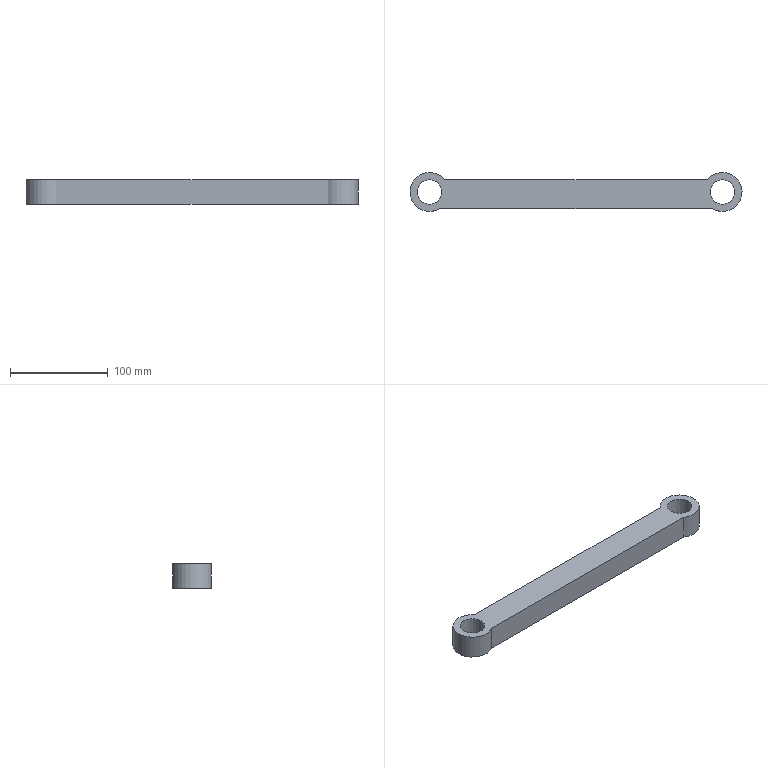Part | NX | features DATUM_CSYS 2, SIMPLE HOLE 2, EXTRUDE 1, HOLE PACKAGE 1, SKETCH 1 | 1 solid | 8 faces | volume 232729 mm3 | cylinder 4 | plane 4 | commonest cylinder face diameters 25 x2 40 x2